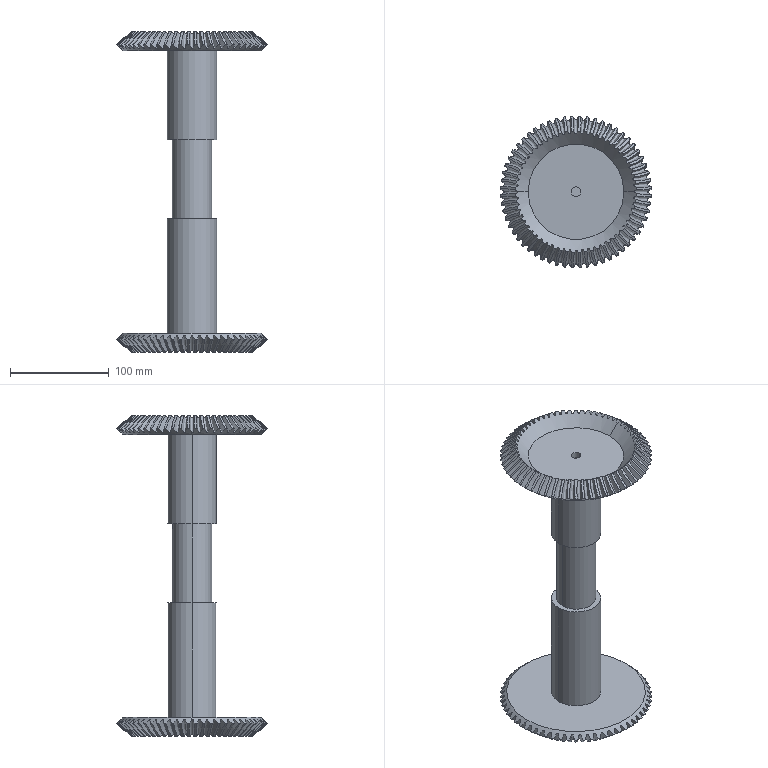Part | SolidWorks | 1 solid | 266 faces | box 153.486 x 153.486 x 325.608 mm | volume 831676 mm3 | cone 128 | spline 120 | cylinder 10 | plane 8 | commonest cylinder face diameters 10 x4 50 x4 40 x2